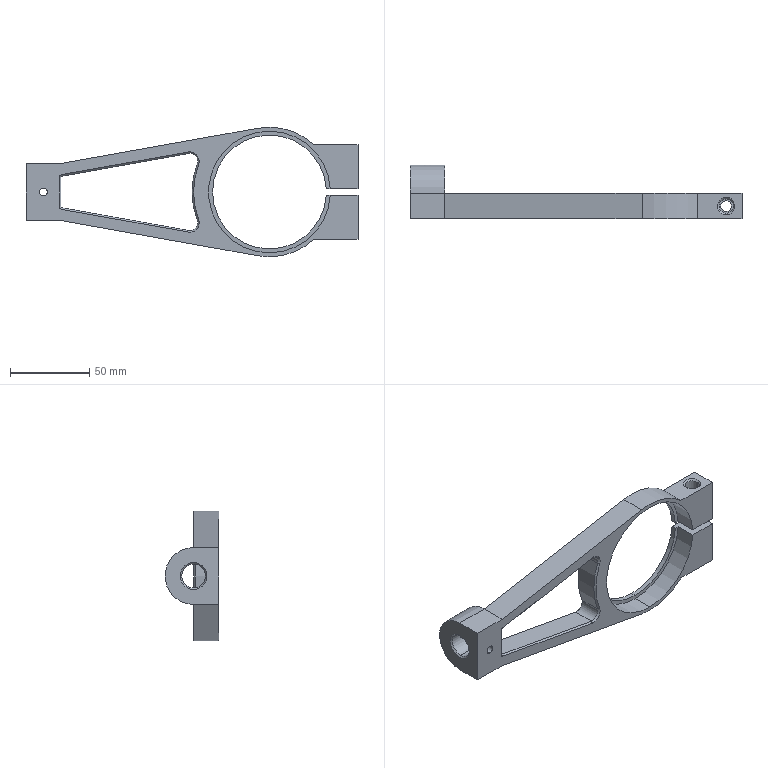Part | SolidWorks | features ICE 6, Chamfer 3, Fillet 2, HoleWzd 2, CutThin 1, ExtruRefSurface 1, Extrusion 1 | 1 solid | 68 faces | box 210 x 34 x 82 mm | volume 81908 mm3 | cylinder 26 | plane 22 | cone 20 | commonest cylinder face diameters 5 x4 10 x3 72 x3 77 x3 82 x3 2 x2